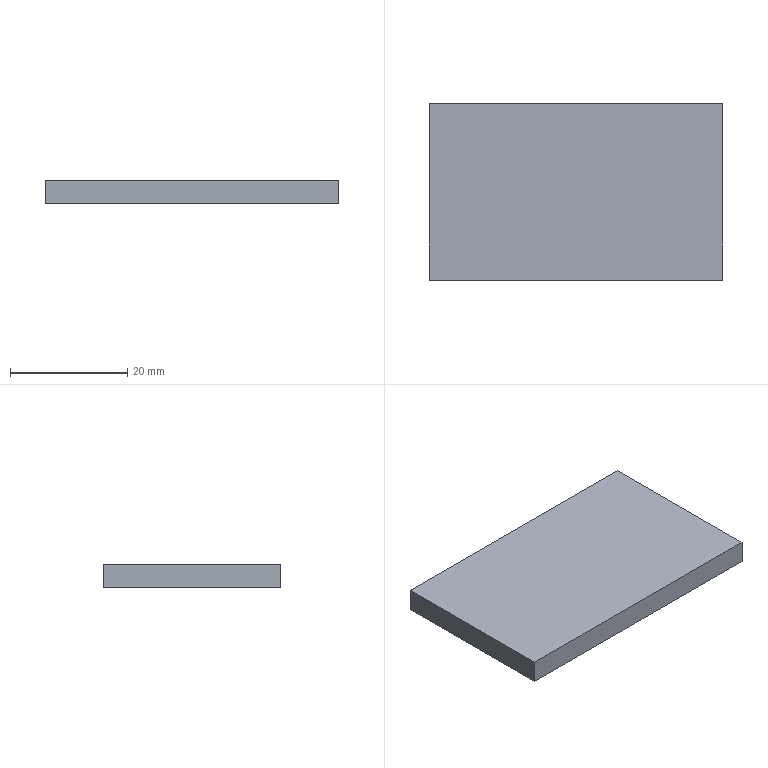Part | STEP file | Q7C0518 | 1 solid | 6 faces | box 50 x 30 x 4 mm | volume 6000 mm3 | plane 6
STEP:
#1=CARTESIAN_POINT('',(0.,0.,0.));
#2=DIRECTION('',(0.,0.,1.));
#3=DIRECTION('',(1.,0.,0.));
#4=AXIS2_PLACEMENT_3D('',#1,#2,#3);
#5=CARTESIAN_POINT('',(25.,-15.,0.));
#6=VERTEX_POINT('',#5);
#7=CARTESIAN_POINT('',(25.,15.,0.));
#8=VERTEX_POINT('',#7);
#9=CARTESIAN_POINT('',(25.,15.,0.));
#10=DIRECTION('',(0.,1.,0.));
#11=VECTOR('',#10,1.);
#12=LINE('',#9,#11);
#13=CARTESIAN_POINT('',(25.,15.,4.));
#14=DIRECTION('',(-1.,0.,0.));
#15=DIRECTION('',(0.,-1.,0.));
#16=AXIS2_PLACEMENT_3D('',#13,#14,#15);
#17=PLANE('',#16);
#18=CARTESIAN_POINT('',(0.,-4.));
#19=DIRECTION('',(-1.,0.));
#20=VECTOR('',#19,1.);
#21=LINE('',#18,#20);
#22=(GEOMETRIC_REPRESENTATION_CONTEXT(2)PARAMETRIC_REPRESENTATION_CONTEXT()REPRESENTATION_CONTEXT('',''));
#23=DEFINITIONAL_REPRESENTATION('',(#21),#22);
#24=PCURVE('',#17,#23);
#25=CARTESIAN_POINT('',(0.,0.,0.));
#26=DIRECTION('',(0.,0.,1.));
#27=DIRECTION('',(1.,0.,0.));
#28=AXIS2_PLACEMENT_3D('',#25,#26,#27);
#29=PLANE('',#28);
#30=CARTESIAN_POINT('',(25.,15.));
#31=DIRECTION('',(0.,1.));
#32=VECTOR('',#31,1.);
#33=LINE('',#30,#32);
#34=(GEOMETRIC_REPRESENTATION_CONTEXT(2)PARAMETRIC_REPRESENTATION_CONTEXT()REPRESENTATION_CONTEXT('',''));
#35=DEFINITIONAL_REPRESENTATION('',(#33),#34);
#36=PCURVE('',#29,#35);
#37=SURFACE_CURVE('',#12,(#24,#36),.PCURVE_S1.);
#38=EDGE_CURVE('',#6,#8,#37,.T.);
#39=ORIENTED_EDGE('',*,*,#38,.T.);
#40=CARTESIAN_POINT('',(25.,15.,4.));
#41=VERTEX_POINT('',#40);
#42=CARTESIAN_POINT('',(25.,15.,4.));
#43=DIRECTION('',(0.,0.,-1.));
#44=VECTOR('',#43,1.);
#45=LINE('',#42,#44);
#46=CARTESIAN_POINT('',(0.,0.));
#47=DIRECTION('',(0.,-1.));
#48=VECTOR('',#47,1.);
#49=LINE('',#46,#48);
#50=(GEOMETRIC_REPRESENTATION_CONTEXT(2)PARAMETRIC_REPRESENTATION_CONTEXT()REPRESENTATION_CONTEXT('',''));
#51=DEFINITIONAL_REPRESENTATION('',(#49),#50);
#52=PCURVE('',#17,#51);
#53=CARTESIAN_POINT('',(-25.,15.,4.));
#54=DIRECTION('',(0.,-1.,0.));
#55=DIRECTION('',(0.,0.,-1.));
#56=AXIS2_PLACEMENT_3D('',#53,#54,#55);
#57=PLANE('',#56);
#58=CARTESIAN_POINT('',(0.,50.));
#59=DIRECTION('',(1.,0.));
#60=VECTOR('',#59,1.);
#61=LINE('',#58,#60);
#62=(GEOMETRIC_REPRESENTATION_CONTEXT(2)PARAMETRIC_REPRESENTATION_CONTEXT()REPRESENTATION_CONTEXT('',''));
#63=DEFINITIONAL_REPRESENTATION('',(#61),#62);
#64=PCURVE('',#57,#63);
#65=SURFACE_CURVE('',#45,(#52,#64),.PCURVE_S1.);
#66=EDGE_CURVE('',#41,#8,#65,.T.);
#67=ORIENTED_EDGE('',*,*,#66,.F.);
#68=CARTESIAN_POINT('',(25.,-15.,4.));
#69=VERTEX_POINT('',#68);
#70=CARTESIAN_POINT('',(25.,15.,4.));
#71=DIRECTION('',(0.,1.,0.));
#72=VECTOR('',#71,1.);
#73=LINE('',#70,#72);
#74=CARTESIAN_POINT('',(0.,0.));
#75=DIRECTION('',(-1.,0.));
#76=VECTOR('',#75,1.);
#77=LINE('',#74,#76);
#78=(GEOMETRIC_REPRESENTATION_CONTEXT(2)PARAMETRIC_REPRESENTATION_CONTEXT()REPRESENTATION_CONTEXT('',''));
#79=DEFINITIONAL_REPRESENTATION('',(#77),#78);
#80=PCURVE('',#17,#79);
#81=CARTESIAN_POINT('',(0.,0.,4.));
#82=DIRECTION('',(0.,0.,1.));
#83=DIRECTION('',(1.,0.,0.));
#84=AXIS2_PLACEMENT_3D('',#81,#82,#83);
#85=PLANE('',#84);
#86=CARTESIAN_POINT('',(25.,15.));
#87=DIRECTION('',(0.,1.));
#88=VECTOR('',#87,1.);
#89=LINE('',#86,#88);
#90=(GEOMETRIC_REPRESENTATION_CONTEXT(2)PARAMETRIC_REPRESENTATION_CONTEXT()REPRESENTATION_CONTEXT('',''));
#91=DEFINITIONAL_REPRESENTATION('',(#89),#90);
#92=PCURVE('',#85,#91);
#93=SURFACE_CURVE('',#73,(#80,#92),.PCURVE_S1.);
#94=EDGE_CURVE('',#69,#41,#93,.T.);
#95=ORIENTED_EDGE('',*,*,#94,.F.);
#96=CARTESIAN_POINT('',(25.,-15.,4.));
#97=DIRECTION('',(0.,0.,-1.));
#98=VECTOR('',#97,1.);
#99=LINE('',#96,#98);
#100=CARTESIAN_POINT('',(30.,0.));
#101=DIRECTION('',(0.,-1.));
#102=VECTOR('',#101,1.);
#103=LINE('',#100,#102);
#104=(GEOMETRIC_REPRESENTATION_CONTEXT(2)PARAMETRIC_REPRESENTATION_CONTEXT()REPRESENTATION_CONTEXT('',''));
#105=DEFINITIONAL_REPRESENTATION('',(#103),#104);
#106=PCURVE('',#17,#105);
#107=CARTESIAN_POINT('',(-25.,-15.,4.));
#108=DIRECTION('',(0.,1.,0.));
#109=DIRECTION('',(0.,0.,1.));
#110=AXIS2_PLACEMENT_3D('',#107,#108,#109);
#111=PLANE('',#110);
#112=CARTESIAN_POINT('',(0.,50.));
#113=DIRECTION('',(-1.,0.));
#114=VECTOR('',#113,1.);
#115=LINE('',#112,#114);
#116=(GEOMETRIC_REPRESENTATION_CONTEXT(2)PARAMETRIC_REPRESENTATION_CONTEXT()REPRESENTATION_CONTEXT('',''));
#117=DEFINITIONAL_REPRESENTATION('',(#115),#116);
#118=PCURVE('',#111,#117);
#119=SURFACE_CURVE('',#99,(#106,#118),.PCURVE_S1.);
#120=EDGE_CURVE('',#69,#6,#119,.T.);
#121=ORIENTED_EDGE('',*,*,#120,.T.);
#122=EDGE_LOOP('',(#39,#67,#95,#121));
#123=FACE_BOUND('',#122,.T.);
#124=ADVANCED_FACE('',(#123),#17,.F.);
#125=CARTESIAN_POINT('',(-25.,15.,0.));
#126=VERTEX_POINT('',#125);
#127=CARTESIAN_POINT('',(-25.,15.,0.));
#128=DIRECTION('',(-1.,0.,0.));
#129=VECTOR('',#128,1.);
#130=LINE('',#127,#129);
#131=CARTESIAN_POINT('',(4.,0.));
#132=DIRECTION('',(0.,-1.));
#133=VECTOR('',#132,1.);
#134=LINE('',#131,#133);
#135=(GEOMETRIC_REPRESENTATION_CONTEXT(2)PARAMETRIC_REPRESENTATION_CONTEXT()REPRESENTATION_CONTEXT('',''));
#136=DEFINITIONAL_REPRESENTATION('',(#134),#135);
#137=PCURVE('',#57,#136);
#138=CARTESIAN_POINT('',(-25.,15.));
#139=DIRECTION('',(-1.,0.));
#140=VECTOR('',#139,1.);
#141=LINE('',#138,#140);
#142=(GEOMETRIC_REPRESENTATION_CONTEXT(2)PARAMETRIC_REPRESENTATION_CONTEXT()REPRESENTATION_CONTEXT('',''));
#143=DEFINITIONAL_REPRESENTATION('',(#141),#142);
#144=PCURVE('',#29,#143);
#145=SURFACE_CURVE('',#130,(#137,#144),.PCURVE_S1.);
#146=EDGE_CURVE('',#8,#126,#145,.T.);
#147=ORIENTED_EDGE('',*,*,#146,.T.);
#148=CARTESIAN_POINT('',(-25.,15.,4.));
#149=VERTEX_POINT('',#148);
#150=CARTESIAN_POINT('',(-25.,15.,4.));
#151=DIRECTION('',(0.,0.,-1.));
#152=VECTOR('',#151,1.);
#153=LINE('',#150,#152);
#154=CARTESIAN_POINT('',(0.,0.));
#155=DIRECTION('',(1.,0.));
#156=VECTOR('',#155,1.);
#157=LINE('',#154,#156);
#158=(GEOMETRIC_REPRESENTATION_CONTEXT(2)PARAMETRIC_REPRESENTATION_CONTEXT()REPRESENTATION_CONTEXT('',''));
#159=DEFINITIONAL_REPRESENTATION('',(#157),#158);
#160=PCURVE('',#57,#159);
#161=CARTESIAN_POINT('',(-25.,15.,4.));
#162=DIRECTION('',(1.,0.,0.));
#163=DIRECTION('',(0.,1.,0.));
#164=AXIS2_PLACEMENT_3D('',#161,#162,#163);
#165=PLANE('',#164);
#166=CARTESIAN_POINT('',(0.,0.));
#167=DIRECTION('',(0.,-1.));
#168=VECTOR('',#167,1.);
#169=LINE('',#166,#168);
#170=(GEOMETRIC_REPRESENTATION_CONTEXT(2)PARAMETRIC_REPRESENTATION_CONTEXT()REPRESENTATION_CONTEXT('',''));
#171=DEFINITIONAL_REPRESENTATION('',(#169),#170);
#172=PCURVE('',#165,#171);
#173=SURFACE_CURVE('',#153,(#160,#172),.PCURVE_S1.);
#174=EDGE_CURVE('',#149,#126,#173,.T.);
#175=ORIENTED_EDGE('',*,*,#174,.F.);
#176=CARTESIAN_POINT('',(-25.,15.,4.));
#177=DIRECTION('',(-1.,0.,0.));
#178=VECTOR('',#177,1.);
#179=LINE('',#176,#178);
#180=CARTESIAN_POINT('',(0.,0.));
#181=DIRECTION('',(0.,-1.));
#182=VECTOR('',#181,1.);
#183=LINE('',#180,#182);
#184=(GEOMETRIC_REPRESENTATION_CONTEXT(2)PARAMETRIC_REPRESENTATION_CONTEXT()REPRESENTATION_CONTEXT('',''));
#185=DEFINITIONAL_REPRESENTATION('',(#183),#184);
#186=PCURVE('',#57,#185);
#187=CARTESIAN_POINT('',(-25.,15.));
#188=DIRECTION('',(-1.,0.));
#189=VECTOR('',#188,1.);
#190=LINE('',#187,#189);
#191=(GEOMETRIC_REPRESENTATION_CONTEXT(2)PARAMETRIC_REPRESENTATION_CONTEXT()REPRESENTATION_CONTEXT('',''));
#192=DEFINITIONAL_REPRESENTATION('',(#190),#191);
#193=PCURVE('',#85,#192);
#194=SURFACE_CURVE('',#179,(#186,#193),.PCURVE_S1.);
#195=EDGE_CURVE('',#41,#149,#194,.T.);
#196=ORIENTED_EDGE('',*,*,#195,.F.);
#197=ORIENTED_EDGE('',*,*,#66,.T.);
#198=EDGE_LOOP('',(#147,#175,#196,#197));
#199=FACE_BOUND('',#198,.T.);
#200=ADVANCED_FACE('',(#199),#57,.F.);
#201=CARTESIAN_POINT('',(-25.,-15.,0.));
#202=VERTEX_POINT('',#201);
#203=CARTESIAN_POINT('',(-25.,15.,0.));
#204=DIRECTION('',(0.,-1.,0.));
#205=VECTOR('',#204,1.);
#206=LINE('',#203,#205);
#207=CARTESIAN_POINT('',(0.,-4.));
#208=DIRECTION('',(-1.,0.));
#209=VECTOR('',#208,1.);
#210=LINE('',#207,#209);
#211=(GEOMETRIC_REPRESENTATION_CONTEXT(2)PARAMETRIC_REPRESENTATION_CONTEXT()REPRESENTATION_CONTEXT('',''));
#212=DEFINITIONAL_REPRESENTATION('',(#210),#211);
#213=PCURVE('',#165,#212);
#214=CARTESIAN_POINT('',(-25.,15.));
#215=DIRECTION('',(0.,-1.));
#216=VECTOR('',#215,1.);
#217=LINE('',#214,#216);
#218=(GEOMETRIC_REPRESENTATION_CONTEXT(2)PARAMETRIC_REPRESENTATION_CONTEXT()REPRESENTATION_CONTEXT('',''));
#219=DEFINITIONAL_REPRESENTATION('',(#217),#218);
#220=PCURVE('',#29,#219);
#221=SURFACE_CURVE('',#206,(#213,#220),.PCURVE_S1.);
#222=EDGE_CURVE('',#126,#202,#221,.T.);
#223=ORIENTED_EDGE('',*,*,#222,.T.);
#224=CARTESIAN_POINT('',(-25.,-15.,4.));
#225=VERTEX_POINT('',#224);
#226=CARTESIAN_POINT('',(-25.,-15.,4.));
#227=DIRECTION('',(0.,0.,-1.));
#228=VECTOR('',#227,1.);
#229=LINE('',#226,#228);
#230=CARTESIAN_POINT('',(-30.,0.));
#231=DIRECTION('',(0.,-1.));
#232=VECTOR('',#231,1.);
#233=LINE('',#230,#232);
#234=(GEOMETRIC_REPRESENTATION_CONTEXT(2)PARAMETRIC_REPRESENTATION_CONTEXT()REPRESENTATION_CONTEXT('',''));
#235=DEFINITIONAL_REPRESENTATION('',(#233),#234);
#236=PCURVE('',#165,#235);
#237=CARTESIAN_POINT('',(0.,0.));
#238=DIRECTION('',(-1.,0.));
#239=VECTOR('',#238,1.);
#240=LINE('',#237,#239);
#241=(GEOMETRIC_REPRESENTATION_CONTEXT(2)PARAMETRIC_REPRESENTATION_CONTEXT()REPRESENTATION_CONTEXT('',''));
#242=DEFINITIONAL_REPRESENTATION('',(#240),#241);
#243=PCURVE('',#111,#242);
#244=SURFACE_CURVE('',#229,(#236,#243),.PCURVE_S1.);
#245=EDGE_CURVE('',#225,#202,#244,.T.);
#246=ORIENTED_EDGE('',*,*,#245,.F.);
#247=CARTESIAN_POINT('',(-25.,15.,4.));
#248=DIRECTION('',(0.,-1.,0.));
#249=VECTOR('',#248,1.);
#250=LINE('',#247,#249);
#251=CARTESIAN_POINT('',(0.,0.));
#252=DIRECTION('',(-1.,0.));
#253=VECTOR('',#252,1.);
#254=LINE('',#251,#253);
#255=(GEOMETRIC_REPRESENTATION_CONTEXT(2)PARAMETRIC_REPRESENTATION_CONTEXT()REPRESENTATION_CONTEXT('',''));
#256=DEFINITIONAL_REPRESENTATION('',(#254),#255);
#257=PCURVE('',#165,#256);
#258=CARTESIAN_POINT('',(-25.,15.));
#259=DIRECTION('',(0.,-1.));
#260=VECTOR('',#259,1.);
#261=LINE('',#258,#260);
#262=(GEOMETRIC_REPRESENTATION_CONTEXT(2)PARAMETRIC_REPRESENTATION_CONTEXT()REPRESENTATION_CONTEXT('',''));
#263=DEFINITIONAL_REPRESENTATION('',(#261),#262);
#264=PCURVE('',#85,#263);
#265=SURFACE_CURVE('',#250,(#257,#264),.PCURVE_S1.);
#266=EDGE_CURVE('',#149,#225,#265,.T.);
#267=ORIENTED_EDGE('',*,*,#266,.F.);
#268=ORIENTED_EDGE('',*,*,#174,.T.);
#269=EDGE_LOOP('',(#223,#246,#267,#268));
#270=FACE_BOUND('',#269,.T.);
#271=ADVANCED_FACE('',(#270),#165,.F.);
#272=CARTESIAN_POINT('',(-25.,-15.,0.));
#273=DIRECTION('',(1.,0.,0.));
#274=VECTOR('',#273,1.);
#275=LINE('',#272,#274);
#276=CARTESIAN_POINT('',(-4.,0.));
#277=DIRECTION('',(0.,1.));
#278=VECTOR('',#277,1.);
#279=LINE('',#276,#278);
#280=(GEOMETRIC_REPRESENTATION_CONTEXT(2)PARAMETRIC_REPRESENTATION_CONTEXT()REPRESENTATION_CONTEXT('',''));
#281=DEFINITIONAL_REPRESENTATION('',(#279),#280);
#282=PCURVE('',#111,#281);
#283=CARTESIAN_POINT('',(-25.,-15.));
#284=DIRECTION('',(1.,0.));
#285=VECTOR('',#284,1.);
#286=LINE('',#283,#285);
#287=(GEOMETRIC_REPRESENTATION_CONTEXT(2)PARAMETRIC_REPRESENTATION_CONTEXT()REPRESENTATION_CONTEXT('',''));
#288=DEFINITIONAL_REPRESENTATION('',(#286),#287);
#289=PCURVE('',#29,#288);
#290=SURFACE_CURVE('',#275,(#282,#289),.PCURVE_S1.);
#291=EDGE_CURVE('',#202,#6,#290,.T.);
#292=ORIENTED_EDGE('',*,*,#291,.T.);
#293=ORIENTED_EDGE('',*,*,#120,.F.);
#294=CARTESIAN_POINT('',(-25.,-15.,4.));
#295=DIRECTION('',(1.,0.,0.));
#296=VECTOR('',#295,1.);
#297=LINE('',#294,#296);
#298=CARTESIAN_POINT('',(0.,0.));
#299=DIRECTION('',(0.,1.));
#300=VECTOR('',#299,1.);
#301=LINE('',#298,#300);
#302=(GEOMETRIC_REPRESENTATION_CONTEXT(2)PARAMETRIC_REPRESENTATION_CONTEXT()REPRESENTATION_CONTEXT('',''));
#303=DEFINITIONAL_REPRESENTATION('',(#301),#302);
#304=PCURVE('',#111,#303);
#305=CARTESIAN_POINT('',(-25.,-15.));
#306=DIRECTION('',(1.,0.));
#307=VECTOR('',#306,1.);
#308=LINE('',#305,#307);
#309=(GEOMETRIC_REPRESENTATION_CONTEXT(2)PARAMETRIC_REPRESENTATION_CONTEXT()REPRESENTATION_CONTEXT('',''));
#310=DEFINITIONAL_REPRESENTATION('',(#308),#309);
#311=PCURVE('',#85,#310);
#312=SURFACE_CURVE('',#297,(#304,#311),.PCURVE_S1.);
#313=EDGE_CURVE('',#225,#69,#312,.T.);
#314=ORIENTED_EDGE('',*,*,#313,.F.);
#315=ORIENTED_EDGE('',*,*,#245,.T.);
#316=EDGE_LOOP('',(#292,#293,#314,#315));
#317=FACE_BOUND('',#316,.T.);
#318=ADVANCED_FACE('',(#317),#111,.F.);
#319=ORIENTED_EDGE('',*,*,#94,.T.);
#320=ORIENTED_EDGE('',*,*,#195,.T.);
#321=ORIENTED_EDGE('',*,*,#266,.T.);
#322=ORIENTED_EDGE('',*,*,#313,.T.);
#323=EDGE_LOOP('',(#319,#320,#321,#322));
#324=FACE_BOUND('',#323,.T.);
#325=ADVANCED_FACE('',(#324),#85,.T.);
#326=ORIENTED_EDGE('',*,*,#38,.F.);
#327=ORIENTED_EDGE('',*,*,#291,.F.);
#328=ORIENTED_EDGE('',*,*,#222,.F.);
#329=ORIENTED_EDGE('',*,*,#146,.F.);
#330=EDGE_LOOP('',(#326,#327,#328,#329));
#331=FACE_BOUND('',#330,.T.);
#332=ADVANCED_FACE('',(#331),#29,.F.);
#333=CLOSED_SHELL('',(#124,#200,#271,#318,#325,#332));
#334=MANIFOLD_SOLID_BREP('',#333);
#335=(LENGTH_UNIT()NAMED_UNIT(*)SI_UNIT(.MILLI.,.METRE.));
#336=UNCERTAINTY_MEASURE_WITH_UNIT(LENGTH_MEASURE(0.0000001),#335,'','');
#337=(NAMED_UNIT(*)PLANE_ANGLE_UNIT()SI_UNIT($,.RADIAN.));
#338=(NAMED_UNIT(*)SI_UNIT($,.STERADIAN.)SOLID_ANGLE_UNIT());
#339=(GEOMETRIC_REPRESENTATION_CONTEXT(3)GLOBAL_UNCERTAINTY_ASSIGNED_CONTEXT((#336))GLOBAL_UNIT_ASSIGNED_CONTEXT((#335,#337,#338))REPRESENTATION_CONTEXT('',''));
#340=ADVANCED_BREP_SHAPE_REPRESENTATION('',(#4,#334),#339);